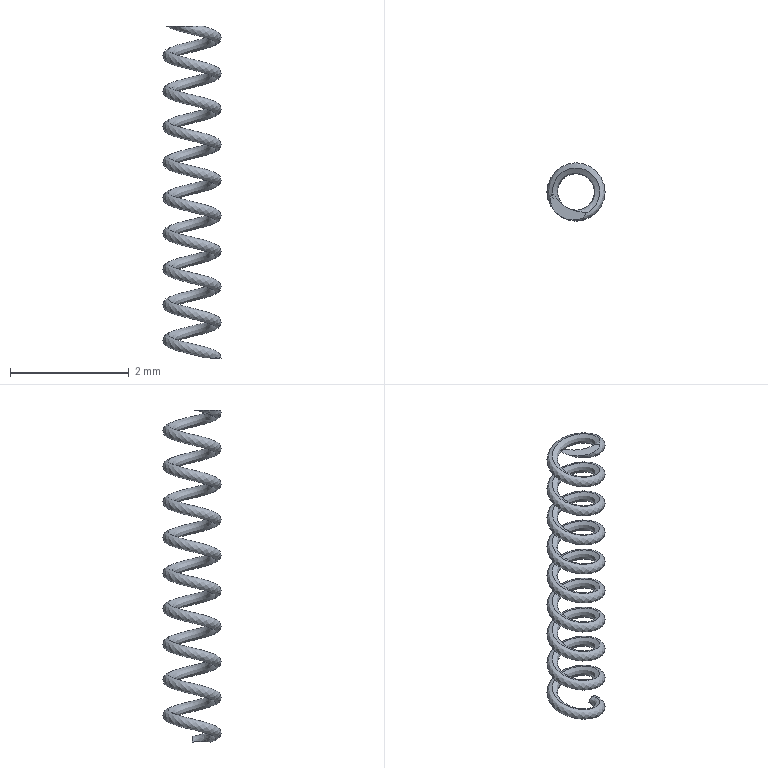Part | SolidWorks | features ICE 2, Helix 1, Sweep 1 | 1 solid | 5 faces | box 0.98 x 0.98 x 5.6 mm | volume 0.5935 mm3 | plane 3 | spline 2